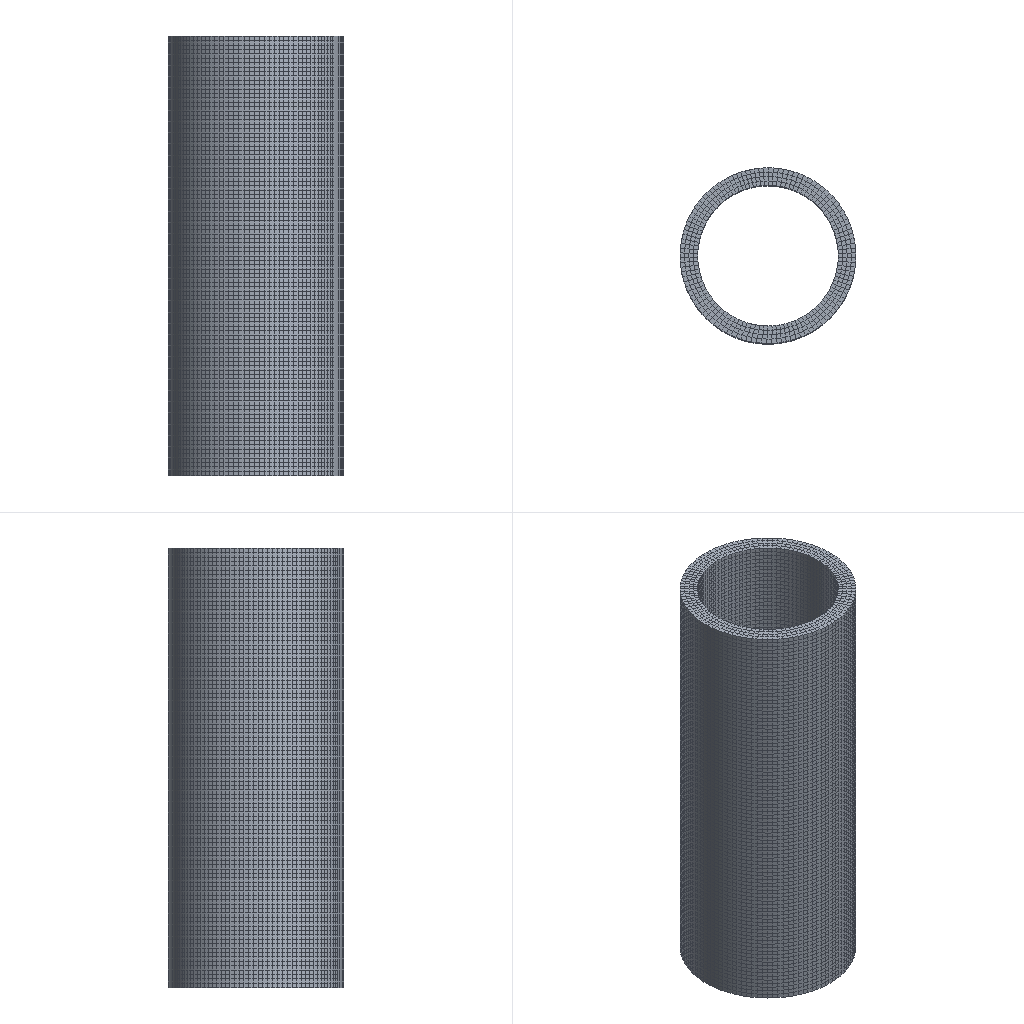Simulation study | abaqus
Set-up summary:
category,name,step,type,value,unit,region
solver,abaqus
solver,version,,,Abaqus/Standard 2020
units,not stated in the deck,,not stated
analysis,deck,,static,static
load_step,Step-1,Step-1,static
load_step,requested,,,1
mesh,nodes,,,56055
mesh,elements,,,44400
element_type,C3D8R,,solid,44400
load,load commands in deck,,count,1
bc,support commands in deck,,count,1
material,MATERIAL-IN,,in results
material,MATERIAL-OUT,,in results
check,setup vs results,,match,"per instance, exact: element labels, types and connectivity; labels of the nodes the elements use; coordinates of those nodes at SINGLE_PRECISION in 1 of 1 instance(s)"
Abaqus input file, long lists of numbers shortened:
*Heading
** Job name: Job-2 Model name: Model-1-Copy
** Generated by: Abaqus/CAE 2020
*Preprint, echo=NO, model=NO, history=NO, contact=NO
**
** PARTS
**
*Part, name=Part-1
*Node
      1,           0.,         -16.,           0.
      2,           0.,         -18.,           0.
** (56053 more lines like these left out)
*Element, type=C3D8R
    1,   960, 34078, 34084,   959,   187,   667,   673,   186
    2, 34078, 11918, 11919, 34084,   667,    46,    47,   673
** (44398 more lines like these left out)
*Nset, nset=Set-1, generate
     1,  56055,      1
*Elset, elset=Set-1, generate
     1,  44400,      1
*Nset, nset=Set-3
     2,     3,     5,     6,     7,     8,     9,    10,    11,    12,    13,    14,    15,    16,    17,    18
    19,    20,    21,    22,    23,    24,    25,    26,    27,    28,    29,    30,    31,    32,    33,    34
** (2101 more lines like these left out)
*Elset, elset=Set-3, generate
 22201,  44400,      1
*Nset, nset=Set-4
     1,     2,     3,     4,     7,     8,     9,    10,    11,    12,    13,    14,    15,    16,    17,    18
    19,    20,    21,    22,    23,    24,    25,    26,    27,    28,    29,    30,    31,    32,    33,    34
** (2101 more lines like these left out)
*Elset, elset=Set-4, generate
     1,  22200,      1
*Nset, nset=Set-6
     2,     3,     5,     6,     7,     8,     9,    10,    11,    12,    13,    14,    15,    16,    17,    18
    19,    20,    21,    22,    23,    24,    25,    26,    27,    28,    29,    30,    31,    32,    33,    34
** (2101 more lines like these left out)
*Elset, elset=Set-6, generate
 22201,  44400,      1
** Section: Section-in
*Solid Section, elset=Set-4, material=Material-in
,
** Section: Section-3
*Solid Section, elset=Set-6, material=Material-out
,
*End Part
**
**
** ASSEMBLY
**
*Assembly, name=Assembly
**
*Instance, name=Part-1-1, part=Part-1
*End Instance
**
*Nset, nset=Set-2, instance=Part-1-1
     1,     2,     3,     4,     5,     6,     7,     8,     9,    10,    11,    12,    13,    14,    15,    16
    17,    18,    19,    20,    21,    22,    23,    24,    25,    26,    27,    28,    29,    30,    31,    32
** (68 more lines like these left out)
*Elset, elset=Set-2, instance=Part-1-1
     1,     2,     3,     4,     5,     6,     7,     8,     9,    10,    11,    12,    13,    14,    15,    16
    17,    18,    19,    20,    21,    22,    23,    24,    25,    26,    27,    28,    29,    30,    31,    32
** (54 more lines like these left out)
*Elset, elset=_Surf-1_S6, internal, instance=Part-1-1
     1,     3,     5,     7,     9,    11,    13,    15,    17,    19,    21,    23,    25,    27,    29,    31
    33,    35,    37,    39,    41,    43,    45,    47,    49,    51,    53,    55,    57,    59,    61,    63
** (405 more lines like these left out)
*Elset, elset=_Surf-1_S4, internal, instance=Part-1-1
    68,    70,    72,    74,    76,    78,    80,    82,    84,    86,    88,    90,    92,    94,    96,    98
   100,   102,   104,   106,   108,   110,   112,   114,   116,   118,   120,   122,   124,   126,   128,   130
** (286 more lines like these left out)
*Surface, type=ELEMENT, name=Surf-1
_Surf-1_S6, S6
_Surf-1_S4, S4
*Elset, elset=_Surf-2_S6, internal, instance=Part-1-1
     1,     3,     5,     7,     9,    11,    13,    15,    17,    19,    21,    23,    25,    27,    29,    31
    33,    35,    37,    39,    41,    43,    45,    47,    49,    51,    53,    55,    57,    59,    61,    63
** (405 more lines like these left out)
*Elset, elset=_Surf-2_S4, internal, instance=Part-1-1
    68,    70,    72,    74,    76,    78,    80,    82,    84,    86,    88,    90,    92,    94,    96,    98
   100,   102,   104,   106,   108,   110,   112,   114,   116,   118,   120,   122,   124,   126,   128,   130
** (286 more lines like these left out)
*Surface, type=ELEMENT, name=Surf-2
_Surf-2_S6, S6
_Surf-2_S4, S4
*End Assembly
**
** MATERIALS
**
*Material, name=Material-in
*Elastic
 3.5, 0.4
*Material, name=Material-out
*Elastic
 0.5, 0.49
** ----------------------------------------------------------------
**
** STEP: Step-1
**
*Step, name=Step-1, nlgeom=YES, inc=1000
*Static, stabilize=0.0002, allsdtol=0.05, continue=NO
0.01, 1., 1e-05, 1.
**
** BOUNDARY CONDITIONS
**
** Name: BC-1 Type: 位移/转角
*Boundary
Set-2, 3, 3
**
** LOADS
**
** Name: Load-1   Type: Pressure
*Dsload
Surf-2, P, 0.01
**
** OUTPUT REQUESTS
**
*Restart, write, frequency=0
**
** FIELD OUTPUT: F-Output-1
**
*Output, field
*Node Output
CF, RF, RM, RT, U, V
*Element Output, directions=YES
E, LE, MISES, MISESMAX, MISESONLY, PE, PEEQ, PEEQMAX, PEEQT, PEMAG, S, SSAVG
*Contact Output
CDISP, CSTRESS
**
** HISTORY OUTPUT: H-Output-1
**
*Output, history, variable=PRESELECT
*End Step
Results summary:
result,step,,completed,increments=11 time=1.0/1.0
result,analysis,,,static
result,last_loadstep,,,1
result,primary field,,,U
result,reaction total,,FX,0.0,model units
result,reaction total,,FY,0.0,model units
result,reaction total,,FZ,0.0,model units